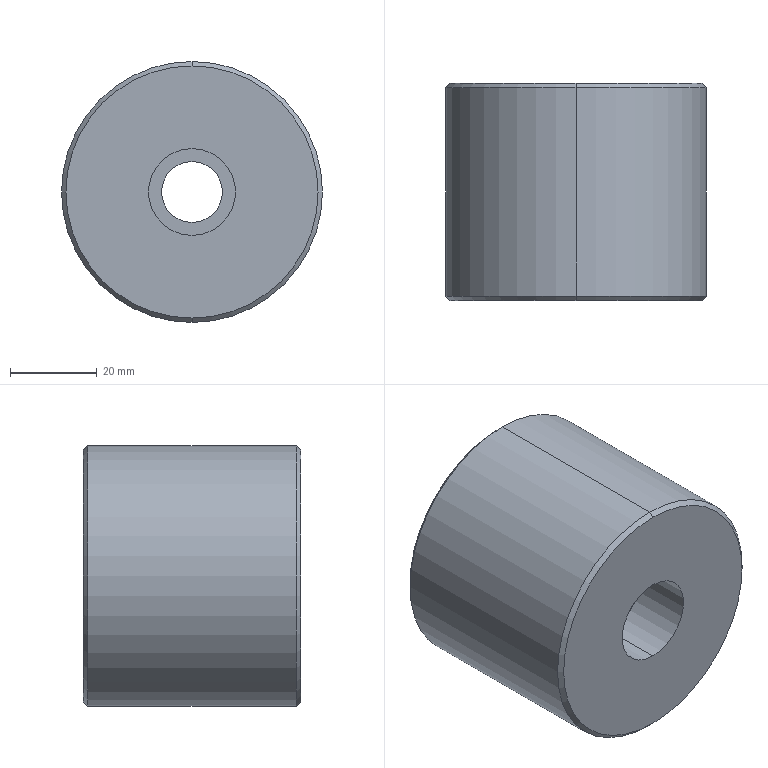Part | Creo | 1 solid | 13 faces | box 60 x 50 x 60 mm | volume 131245 mm3 | cylinder 6 | cone 4 | plane 3 | commonest cylinder face diameters 14 x2 20 x2 60 x2
STEP:
#1=CARTESIAN_POINT('',(-244.,-401.,-312.));
#2=VERTEX_POINT('',#1);
#3=CARTESIAN_POINT('',(-244.,-401.,-254.));
#4=VERTEX_POINT('',#3);
#5=CARTESIAN_POINT('',(-244.,-401.,-283.));
#6=DIRECTION('',(0.,-1.,0.));
#7=DIRECTION('',(0.,0.,-1.));
#8=AXIS2_PLACEMENT_3D('',#5,#6,#7);
#9=CIRCLE('',#8,29.);
#10=EDGE_CURVE('',#2,#4,#9,.T.);
#11=ORIENTED_EDGE('',*,*,#10,.F.);
#12=CARTESIAN_POINT('',(-244.,-401.,-283.));
#13=DIRECTION('',(0.,-1.,0.));
#14=DIRECTION('',(0.,0.,1.));
#15=AXIS2_PLACEMENT_3D('',#12,#13,#14);
#16=CIRCLE('',#15,29.);
#17=EDGE_CURVE('',#4,#2,#16,.T.);
#18=ORIENTED_EDGE('',*,*,#17,.F.);
#19=EDGE_LOOP('',(#11,#18));
#20=FACE_OUTER_BOUND('',#19,.F.);
#21=CARTESIAN_POINT('',(-244.,-401.,-293.));
#22=VERTEX_POINT('',#21);
#23=CARTESIAN_POINT('',(-244.,-401.,-273.));
#24=VERTEX_POINT('',#23);
#25=CARTESIAN_POINT('',(-244.,-401.,-283.));
#26=DIRECTION('',(0.,1.,0.));
#27=DIRECTION('',(0.,0.,-1.));
#28=AXIS2_PLACEMENT_3D('',#25,#26,#27);
#29=CIRCLE('',#28,10.);
#30=EDGE_CURVE('',#22,#24,#29,.T.);
#31=ORIENTED_EDGE('',*,*,#30,.F.);
#32=CARTESIAN_POINT('',(-244.,-401.,-283.));
#33=DIRECTION('',(0.,1.,0.));
#34=DIRECTION('',(0.,0.,1.));
#35=AXIS2_PLACEMENT_3D('',#32,#33,#34);
#36=CIRCLE('',#35,10.);
#37=EDGE_CURVE('',#24,#22,#36,.T.);
#38=ORIENTED_EDGE('',*,*,#37,.F.);
#39=EDGE_LOOP('',(#31,#38));
#40=FACE_BOUND('',#39,.F.);
#41=CARTESIAN_POINT('',(-244.,-401.,-283.));
#42=DIRECTION('',(0.,-1.,0.));
#43=DIRECTION('',(0.,0.,-1.));
#44=AXIS2_PLACEMENT_3D('',#41,#42,#43);
#45=PLANE('',#44);
#46=ADVANCED_FACE('',(#20,#40),#45,.T.);
#47=ORIENTED_EDGE('',*,*,#10,.T.);
#48=CARTESIAN_POINT('',(-244.,-400.,-253.));
#49=VERTEX_POINT('',#48);
#50=CARTESIAN_POINT('',(-244.,-401.,-254.));
#51=DIRECTION('',(0.,0.7071,0.7071));
#52=VECTOR('',#51,1.414);
#53=LINE('',#50,#52);
#54=EDGE_CURVE('',#4,#49,#53,.T.);
#55=ORIENTED_EDGE('',*,*,#54,.T.);
#56=CARTESIAN_POINT('',(-244.,-400.,-313.));
#57=VERTEX_POINT('',#56);
#58=CARTESIAN_POINT('',(-244.,-400.,-283.));
#59=DIRECTION('',(0.,-1.,0.));
#60=DIRECTION('',(0.,0.,-1.));
#61=AXIS2_PLACEMENT_3D('',#58,#59,#60);
#62=CIRCLE('',#61,30.);
#63=EDGE_CURVE('',#57,#49,#62,.T.);
#64=ORIENTED_EDGE('',*,*,#63,.F.);
#65=CARTESIAN_POINT('',(-244.,-401.,-312.));
#66=DIRECTION('',(0.,0.7071,-0.7071));
#67=VECTOR('',#66,1.414);
#68=LINE('',#65,#67);
#69=EDGE_CURVE('',#2,#57,#68,.T.);
#70=ORIENTED_EDGE('',*,*,#69,.F.);
#71=EDGE_LOOP('',(#47,#55,#64,#70));
#72=FACE_OUTER_BOUND('',#71,.F.);
#73=CARTESIAN_POINT('',(-244.,-400.5,-283.));
#74=DIRECTION('',(0.,1.,0.));
#75=DIRECTION('',(0.,0.,1.));
#76=AXIS2_PLACEMENT_3D('',#73,#74,#75);
#77=CONICAL_SURFACE('',#76,29.5,45.);
#78=ADVANCED_FACE('',(#72),#77,.T.);
#79=ORIENTED_EDGE('',*,*,#17,.T.);
#80=ORIENTED_EDGE('',*,*,#69,.T.);
#81=CARTESIAN_POINT('',(-244.,-400.,-283.));
#82=DIRECTION('',(0.,-1.,0.));
#83=DIRECTION('',(0.,0.,1.));
#84=AXIS2_PLACEMENT_3D('',#81,#82,#83);
#85=CIRCLE('',#84,30.);
#86=EDGE_CURVE('',#49,#57,#85,.T.);
#87=ORIENTED_EDGE('',*,*,#86,.F.);
#88=ORIENTED_EDGE('',*,*,#54,.F.);
#89=EDGE_LOOP('',(#79,#80,#87,#88));
#90=FACE_OUTER_BOUND('',#89,.F.);
#91=CARTESIAN_POINT('',(-244.,-400.5,-283.));
#92=DIRECTION('',(0.,1.,0.));
#93=DIRECTION('',(0.,0.,1.));
#94=AXIS2_PLACEMENT_3D('',#91,#92,#93);
#95=CONICAL_SURFACE('',#94,29.5,45.);
#96=ADVANCED_FACE('',(#90),#95,.T.);
#97=ORIENTED_EDGE('',*,*,#86,.T.);
#98=CARTESIAN_POINT('',(-244.,-352.,-313.));
#99=VERTEX_POINT('',#98);
#100=CARTESIAN_POINT('',(-244.,-352.,-313.));
#101=DIRECTION('',(0.,-1.,0.));
#102=VECTOR('',#101,48.);
#103=LINE('',#100,#102);
#104=EDGE_CURVE('',#99,#57,#103,.T.);
#105=ORIENTED_EDGE('',*,*,#104,.F.);
#106=CARTESIAN_POINT('',(-244.,-352.,-253.));
#107=VERTEX_POINT('',#106);
#108=CARTESIAN_POINT('',(-244.,-352.,-283.));
#109=DIRECTION('',(0.,1.,0.));
#110=DIRECTION('',(0.,0.,-1.));
#111=AXIS2_PLACEMENT_3D('',#108,#109,#110);
#112=CIRCLE('',#111,30.);
#113=EDGE_CURVE('',#99,#107,#112,.T.);
#114=ORIENTED_EDGE('',*,*,#113,.T.);
#115=CARTESIAN_POINT('',(-244.,-352.,-253.));
#116=DIRECTION('',(0.,-1.,0.));
#117=VECTOR('',#116,48.);
#118=LINE('',#115,#117);
#119=EDGE_CURVE('',#107,#49,#118,.T.);
#120=ORIENTED_EDGE('',*,*,#119,.T.);
#121=EDGE_LOOP('',(#97,#105,#114,#120));
#122=FACE_OUTER_BOUND('',#121,.F.);
#123=CARTESIAN_POINT('',(-244.,-351.,-283.));
#124=DIRECTION('',(0.,-1.,0.));
#125=DIRECTION('',(0.,0.,-1.));
#126=AXIS2_PLACEMENT_3D('',#123,#124,#125);
#127=CYLINDRICAL_SURFACE('',#126,30.);
#128=ADVANCED_FACE('',(#122),#127,.T.);
#129=ORIENTED_EDGE('',*,*,#63,.T.);
#130=ORIENTED_EDGE('',*,*,#119,.F.);
#131=CARTESIAN_POINT('',(-244.,-352.,-283.));
#132=DIRECTION('',(0.,1.,0.));
#133=DIRECTION('',(0.,0.,1.));
#134=AXIS2_PLACEMENT_3D('',#131,#132,#133);
#135=CIRCLE('',#134,30.);
#136=EDGE_CURVE('',#107,#99,#135,.T.);
#137=ORIENTED_EDGE('',*,*,#136,.T.);
#138=ORIENTED_EDGE('',*,*,#104,.T.);
#139=EDGE_LOOP('',(#129,#130,#137,#138));
#140=FACE_OUTER_BOUND('',#139,.F.);
#141=CARTESIAN_POINT('',(-244.,-351.,-283.));
#142=DIRECTION('',(0.,-1.,0.));
#143=DIRECTION('',(0.,0.,-1.));
#144=AXIS2_PLACEMENT_3D('',#141,#142,#143);
#145=CYLINDRICAL_SURFACE('',#144,30.);
#146=ADVANCED_FACE('',(#140),#145,.T.);
#147=CARTESIAN_POINT('',(-244.,-351.,-254.));
#148=VERTEX_POINT('',#147);
#149=CARTESIAN_POINT('',(-244.,-351.,-312.));
#150=VERTEX_POINT('',#149);
#151=CARTESIAN_POINT('',(-244.,-351.,-283.));
#152=DIRECTION('',(0.,1.,0.));
#153=DIRECTION('',(0.,0.,1.));
#154=AXIS2_PLACEMENT_3D('',#151,#152,#153);
#155=CIRCLE('',#154,29.);
#156=EDGE_CURVE('',#148,#150,#155,.T.);
#157=ORIENTED_EDGE('',*,*,#156,.T.);
#158=CARTESIAN_POINT('',(-244.,-351.,-312.));
#159=DIRECTION('',(0.,-0.7071,-0.7071));
#160=VECTOR('',#159,1.414);
#161=LINE('',#158,#160);
#162=EDGE_CURVE('',#150,#99,#161,.T.);
#163=ORIENTED_EDGE('',*,*,#162,.T.);
#164=ORIENTED_EDGE('',*,*,#136,.F.);
#165=CARTESIAN_POINT('',(-244.,-351.,-254.));
#166=DIRECTION('',(0.,-0.7071,0.7071));
#167=VECTOR('',#166,1.414);
#168=LINE('',#165,#167);
#169=EDGE_CURVE('',#148,#107,#168,.T.);
#170=ORIENTED_EDGE('',*,*,#169,.F.);
#171=EDGE_LOOP('',(#157,#163,#164,#170));
#172=FACE_OUTER_BOUND('',#171,.F.);
#173=CARTESIAN_POINT('',(-244.,-351.5,-283.));
#174=DIRECTION('',(0.,-1.,0.));
#175=DIRECTION('',(0.,0.,-1.));
#176=AXIS2_PLACEMENT_3D('',#173,#174,#175);
#177=CONICAL_SURFACE('',#176,29.5,45.);
#178=ADVANCED_FACE('',(#172),#177,.T.);
#179=ORIENTED_EDGE('',*,*,#156,.F.);
#180=CARTESIAN_POINT('',(-244.,-351.,-283.));
#181=DIRECTION('',(0.,1.,0.));
#182=DIRECTION('',(0.,0.,-1.));
#183=AXIS2_PLACEMENT_3D('',#180,#181,#182);
#184=CIRCLE('',#183,29.);
#185=EDGE_CURVE('',#150,#148,#184,.T.);
#186=ORIENTED_EDGE('',*,*,#185,.F.);
#187=EDGE_LOOP('',(#179,#186));
#188=FACE_OUTER_BOUND('',#187,.F.);
#189=CARTESIAN_POINT('',(-244.,-351.,-276.));
#190=VERTEX_POINT('',#189);
#191=CARTESIAN_POINT('',(-244.,-351.,-290.));
#192=VERTEX_POINT('',#191);
#193=CARTESIAN_POINT('',(-244.,-351.,-283.));
#194=DIRECTION('',(0.,-1.,0.));
#195=DIRECTION('',(0.,0.,1.));
#196=AXIS2_PLACEMENT_3D('',#193,#194,#195);
#197=CIRCLE('',#196,7.);
#198=EDGE_CURVE('',#190,#192,#197,.T.);
#199=ORIENTED_EDGE('',*,*,#198,.F.);
#200=CARTESIAN_POINT('',(-244.,-351.,-283.));
#201=DIRECTION('',(0.,-1.,0.));
#202=DIRECTION('',(0.,0.,-1.));
#203=AXIS2_PLACEMENT_3D('',#200,#201,#202);
#204=CIRCLE('',#203,7.);
#205=EDGE_CURVE('',#192,#190,#204,.T.);
#206=ORIENTED_EDGE('',*,*,#205,.F.);
#207=EDGE_LOOP('',(#199,#206));
#208=FACE_BOUND('',#207,.F.);
#209=CARTESIAN_POINT('',(-244.,-351.,-283.));
#210=DIRECTION('',(0.,1.,0.));
#211=DIRECTION('',(0.,0.,1.));
#212=AXIS2_PLACEMENT_3D('',#209,#210,#211);
#213=PLANE('',#212);
#214=ADVANCED_FACE('',(#188,#208),#213,.T.);
#215=ORIENTED_EDGE('',*,*,#185,.T.);
#216=ORIENTED_EDGE('',*,*,#169,.T.);
#217=ORIENTED_EDGE('',*,*,#113,.F.);
#218=ORIENTED_EDGE('',*,*,#162,.F.);
#219=EDGE_LOOP('',(#215,#216,#217,#218));
#220=FACE_OUTER_BOUND('',#219,.F.);
#221=CARTESIAN_POINT('',(-244.,-351.5,-283.));
#222=DIRECTION('',(0.,-1.,0.));
#223=DIRECTION('',(0.,0.,-1.));
#224=AXIS2_PLACEMENT_3D('',#221,#222,#223);
#225=CONICAL_SURFACE('',#224,29.5,45.);
#226=ADVANCED_FACE('',(#220),#225,.T.);
#227=CARTESIAN_POINT('',(-244.,-387.,-290.));
#228=VERTEX_POINT('',#227);
#229=CARTESIAN_POINT('',(-244.,-387.,-276.));
#230=VERTEX_POINT('',#229);
#231=CARTESIAN_POINT('',(-244.,-387.,-283.));
#232=DIRECTION('',(0.,1.,0.));
#233=DIRECTION('',(0.,0.,-1.));
#234=AXIS2_PLACEMENT_3D('',#231,#232,#233);
#235=CIRCLE('',#234,7.);
#236=EDGE_CURVE('',#228,#230,#235,.T.);
#237=ORIENTED_EDGE('',*,*,#236,.T.);
#238=CARTESIAN_POINT('',(-244.,-387.,-276.));
#239=DIRECTION('',(0.,1.,0.));
#240=VECTOR('',#239,36.);
#241=LINE('',#238,#240);
#242=EDGE_CURVE('',#230,#190,#241,.T.);
#243=ORIENTED_EDGE('',*,*,#242,.T.);
#244=ORIENTED_EDGE('',*,*,#198,.T.);
#245=CARTESIAN_POINT('',(-244.,-387.,-290.));
#246=DIRECTION('',(0.,1.,0.));
#247=VECTOR('',#246,36.);
#248=LINE('',#245,#247);
#249=EDGE_CURVE('',#228,#192,#248,.T.);
#250=ORIENTED_EDGE('',*,*,#249,.F.);
#251=EDGE_LOOP('',(#237,#243,#244,#250));
#252=FACE_OUTER_BOUND('',#251,.F.);
#253=CARTESIAN_POINT('',(-244.,-401.,-283.));
#254=DIRECTION('',(0.,1.,0.));
#255=DIRECTION('',(0.,0.,-1.));
#256=AXIS2_PLACEMENT_3D('',#253,#254,#255);
#257=CYLINDRICAL_SURFACE('',#256,7.);
#258=ADVANCED_FACE('',(#252),#257,.F.);
#259=CARTESIAN_POINT('',(-244.,-387.,-273.));
#260=VERTEX_POINT('',#259);
#261=CARTESIAN_POINT('',(-244.,-387.,-293.));
#262=VERTEX_POINT('',#261);
#263=CARTESIAN_POINT('',(-244.,-387.,-283.));
#264=DIRECTION('',(0.,-1.,0.));
#265=DIRECTION('',(0.,0.,1.));
#266=AXIS2_PLACEMENT_3D('',#263,#264,#265);
#267=CIRCLE('',#266,10.);
#268=EDGE_CURVE('',#260,#262,#267,.T.);
#269=ORIENTED_EDGE('',*,*,#268,.F.);
#270=CARTESIAN_POINT('',(-244.,-387.,-283.));
#271=DIRECTION('',(0.,-1.,0.));
#272=DIRECTION('',(0.,0.,-1.));
#273=AXIS2_PLACEMENT_3D('',#270,#271,#272);
#274=CIRCLE('',#273,10.);
#275=EDGE_CURVE('',#262,#260,#274,.T.);
#276=ORIENTED_EDGE('',*,*,#275,.F.);
#277=EDGE_LOOP('',(#269,#276));
#278=FACE_OUTER_BOUND('',#277,.F.);
#279=CARTESIAN_POINT('',(-244.,-387.,-283.));
#280=DIRECTION('',(0.,1.,0.));
#281=DIRECTION('',(0.,0.,1.));
#282=AXIS2_PLACEMENT_3D('',#279,#280,#281);
#283=CIRCLE('',#282,7.);
#284=EDGE_CURVE('',#230,#228,#283,.T.);
#285=ORIENTED_EDGE('',*,*,#284,.F.);
#286=ORIENTED_EDGE('',*,*,#236,.F.);
#287=EDGE_LOOP('',(#285,#286));
#288=FACE_BOUND('',#287,.F.);
#289=CARTESIAN_POINT('',(-244.,-387.,-283.));
#290=DIRECTION('',(0.,1.,0.));
#291=DIRECTION('',(0.,0.,-1.));
#292=AXIS2_PLACEMENT_3D('',#289,#290,#291);
#293=PLANE('',#292);
#294=ADVANCED_FACE('',(#278,#288),#293,.F.);
#295=ORIENTED_EDGE('',*,*,#284,.T.);
#296=ORIENTED_EDGE('',*,*,#249,.T.);
#297=ORIENTED_EDGE('',*,*,#205,.T.);
#298=ORIENTED_EDGE('',*,*,#242,.F.);
#299=EDGE_LOOP('',(#295,#296,#297,#298));
#300=FACE_OUTER_BOUND('',#299,.F.);
#301=CARTESIAN_POINT('',(-244.,-401.,-283.));
#302=DIRECTION('',(0.,1.,0.));
#303=DIRECTION('',(0.,0.,-1.));
#304=AXIS2_PLACEMENT_3D('',#301,#302,#303);
#305=CYLINDRICAL_SURFACE('',#304,7.);
#306=ADVANCED_FACE('',(#300),#305,.F.);
#307=ORIENTED_EDGE('',*,*,#268,.T.);
#308=CARTESIAN_POINT('',(-244.,-401.,-293.));
#309=DIRECTION('',(0.,1.,0.));
#310=VECTOR('',#309,14.);
#311=LINE('',#308,#310);
#312=EDGE_CURVE('',#22,#262,#311,.T.);
#313=ORIENTED_EDGE('',*,*,#312,.F.);
#314=ORIENTED_EDGE('',*,*,#30,.T.);
#315=CARTESIAN_POINT('',(-244.,-401.,-273.));
#316=DIRECTION('',(0.,1.,0.));
#317=VECTOR('',#316,14.);
#318=LINE('',#315,#317);
#319=EDGE_CURVE('',#24,#260,#318,.T.);
#320=ORIENTED_EDGE('',*,*,#319,.T.);
#321=EDGE_LOOP('',(#307,#313,#314,#320));
#322=FACE_OUTER_BOUND('',#321,.F.);
#323=CARTESIAN_POINT('',(-244.,-401.,-283.));
#324=DIRECTION('',(0.,1.,0.));
#325=DIRECTION('',(0.,0.,-1.));
#326=AXIS2_PLACEMENT_3D('',#323,#324,#325);
#327=CYLINDRICAL_SURFACE('',#326,10.);
#328=ADVANCED_FACE('',(#322),#327,.F.);
#329=ORIENTED_EDGE('',*,*,#275,.T.);
#330=ORIENTED_EDGE('',*,*,#319,.F.);
#331=ORIENTED_EDGE('',*,*,#37,.T.);
#332=ORIENTED_EDGE('',*,*,#312,.T.);
#333=EDGE_LOOP('',(#329,#330,#331,#332));
#334=FACE_OUTER_BOUND('',#333,.F.);
#335=CARTESIAN_POINT('',(-244.,-401.,-283.));
#336=DIRECTION('',(0.,1.,0.));
#337=DIRECTION('',(0.,0.,-1.));
#338=AXIS2_PLACEMENT_3D('',#335,#336,#337);
#339=CYLINDRICAL_SURFACE('',#338,10.);
#340=ADVANCED_FACE('',(#334),#339,.F.);
#341=CLOSED_SHELL('',(#46,#78,#96,#128,#146,#178,#214,#226,#258,#294,#306,#328,#340));
#342=MANIFOLD_SOLID_BREP('',#341);
#343=(LENGTH_UNIT()NAMED_UNIT(*)SI_UNIT(.MILLI.,.METRE.));
#344=UNCERTAINTY_MEASURE_WITH_UNIT(LENGTH_MEASURE(0.009848),#343,'','');
#345=(NAMED_UNIT(*)PLANE_ANGLE_UNIT()SI_UNIT($,.RADIAN.));
#346=PLANE_ANGLE_MEASURE_WITH_UNIT(PLANE_ANGLE_MEASURE(0.01745),#345);
#347=(CONVERSION_BASED_UNIT('DEGREE',#346)NAMED_UNIT(*)PLANE_ANGLE_UNIT());
#348=(NAMED_UNIT(*)SI_UNIT($,.STERADIAN.)SOLID_ANGLE_UNIT());
#349=(GEOMETRIC_REPRESENTATION_CONTEXT(3)GLOBAL_UNCERTAINTY_ASSIGNED_CONTEXT((#344))GLOBAL_UNIT_ASSIGNED_CONTEXT((#343,#347,#348))REPRESENTATION_CONTEXT('',''));
#350=ADVANCED_BREP_SHAPE_REPRESENTATION('',(#342),#349);